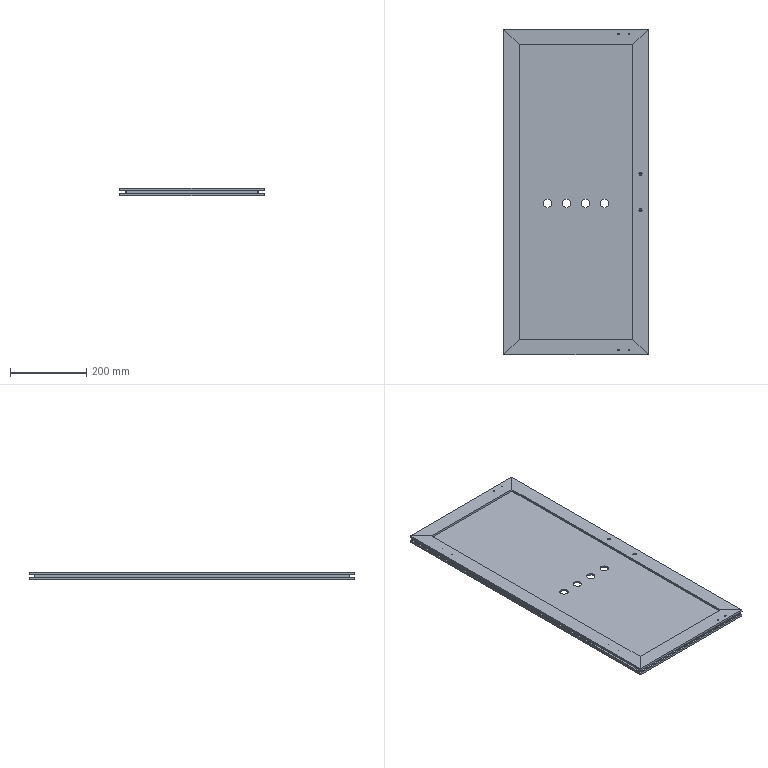Part | SolidWorks | features HoleWzd 3, ICE 3, WeldMemberFeat 1, WeldmentFeature 1 | 6 solids | 198 faces | box 379.5 x 856 x 20 mm | volume 2241124 mm3 | plane 138 | cylinder 52 | cone 8 | commonest cylinder face diameters 5 x16 3.3 x8 4.5 x8 6.5 x8 22 x8 8 x4